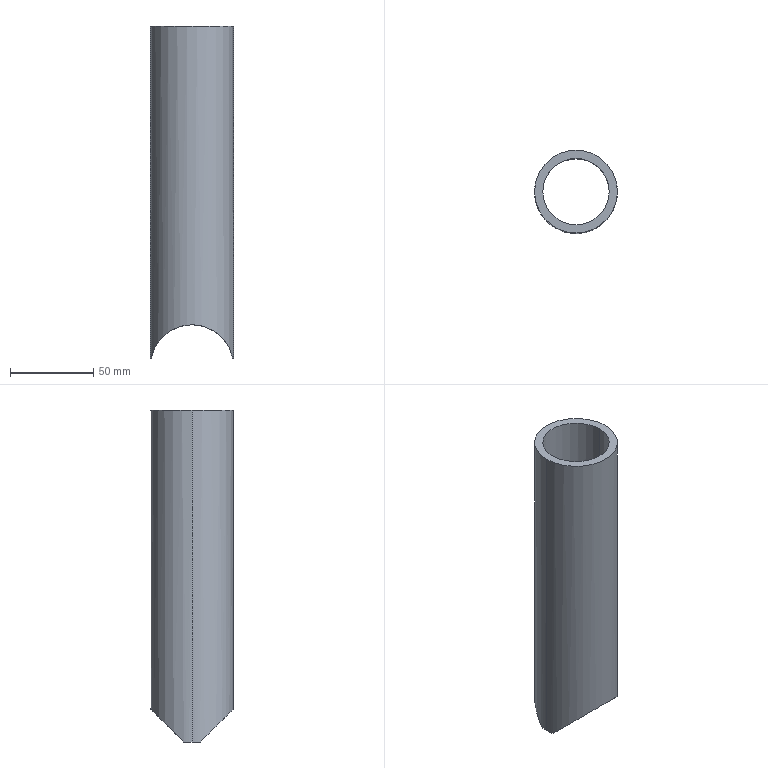Part | SolidWorks | features Extrusion 1, ICE 1, WeldmentFeature 1 | 1 solid | 8 faces | box 50 x 50 x 200 mm | volume 131874 mm3 | cylinder 5 | plane 3 | commonest cylinder face diameters 50 x3 40 x2
STEP:
#1=CARTESIAN_POINT('',(-20.,0.,200.));
#2=VERTEX_POINT('',#1);
#3=CARTESIAN_POINT('',(20.,0.,200.));
#4=VERTEX_POINT('',#3);
#5=CARTESIAN_POINT('',(0.,0.,200.));
#6=DIRECTION('',(0.,0.,1.));
#7=DIRECTION('',(1.,0.,0.));
#8=AXIS2_PLACEMENT_3D('',#5,#6,#7);
#9=CIRCLE('',#8,20.);
#10=EDGE_CURVE('',#2,#4,#9,.T.);
#11=ORIENTED_EDGE('',*,*,#10,.T.);
#12=CARTESIAN_POINT('',(20.,0.,10.));
#13=VERTEX_POINT('',#12);
#14=CARTESIAN_POINT('',(20.,0.,200.));
#15=DIRECTION('',(0.,0.,-1.));
#16=VECTOR('',#15,1000.);
#17=LINE('',#14,#16);
#18=EDGE_CURVE('',#4,#13,#17,.T.);
#19=ORIENTED_EDGE('',*,*,#18,.T.);
#20=CARTESIAN_POINT('',(-20.,0.,10.));
#21=VERTEX_POINT('',#20);
#22=CARTESIAN_POINT('',(20.,0.,10.));
#23=CARTESIAN_POINT('',(20.,-0.6946,10.));
#24=CARTESIAN_POINT('',(19.964,-1.383,10.048));
#25=CARTESIAN_POINT('',(19.858,-2.406,10.188));
#26=CARTESIAN_POINT('',(19.814,-2.745,10.246));
#27=CARTESIAN_POINT('',(19.708,-3.421,10.382));
#28=CARTESIAN_POINT('',(19.647,-3.758,10.46));
#29=CARTESIAN_POINT('',(19.302,-5.409,10.894));
#30=CARTESIAN_POINT('',(18.908,-6.644,11.372));
#31=CARTESIAN_POINT('',(18.158,-8.409,12.188));
#32=CARTESIAN_POINT('',(17.88,-8.983,12.478));
#33=CARTESIAN_POINT('',(17.283,-10.085,13.069));
#34=CARTESIAN_POINT('',(16.962,-10.615,13.372));
#35=CARTESIAN_POINT('',(15.932,-12.154,14.288));
#36=CARTESIAN_POINT('',(15.156,-13.109,14.91));
#37=CARTESIAN_POINT('',(13.845,-14.447,15.823));
#38=CARTESIAN_POINT('',(13.382,-14.877,16.124));
#39=CARTESIAN_POINT('',(12.423,-15.687,16.702));
#40=CARTESIAN_POINT('',(11.924,-16.069,16.981));
#41=CARTESIAN_POINT('',(10.366,-17.151,17.78));
#42=CARTESIAN_POINT('',(9.247,-17.784,18.263));
#43=CARTESIAN_POINT('',(7.725,-18.451,18.779));
#44=CARTESIAN_POINT('',(7.414,-18.578,18.878));
#45=CARTESIAN_POINT('',(6.785,-18.817,19.064));
#46=CARTESIAN_POINT('',(6.468,-18.928,19.151));
#47=CARTESIAN_POINT('',(5.505,-19.239,19.395));
#48=CARTESIAN_POINT('',(4.851,-19.415,19.534));
#49=CARTESIAN_POINT('',(3.517,-19.7,19.761));
#50=CARTESIAN_POINT('',(2.835,-19.81,19.848));
#51=CARTESIAN_POINT('',(1.447,-19.96,19.968));
#52=CARTESIAN_POINT('',(0.7543,-19.998,19.998));
#53=CARTESIAN_POINT('',(-0.6273,-20.002,20.002));
#54=CARTESIAN_POINT('',(-1.316,-19.969,19.975));
#55=CARTESIAN_POINT('',(-2.347,-19.865,19.892));
#56=CARTESIAN_POINT('',(-2.69,-19.821,19.857));
#57=CARTESIAN_POINT('',(-3.376,-19.716,19.773));
#58=CARTESIAN_POINT('',(-3.718,-19.654,19.724));
#59=CARTESIAN_POINT('',(-5.403,-19.306,19.447));
#60=CARTESIAN_POINT('',(-6.686,-18.897,19.124));
#61=CARTESIAN_POINT('',(-8.218,-18.237,18.613));
#62=CARTESIAN_POINT('',(-8.521,-18.097,18.505));
#63=CARTESIAN_POINT('',(-9.114,-17.806,18.282));
#64=CARTESIAN_POINT('',(-9.405,-17.654,18.166));
#65=CARTESIAN_POINT('',(-10.26,-17.18,17.806));
#66=CARTESIAN_POINT('',(-10.807,-16.841,17.551));
#67=CARTESIAN_POINT('',(-11.862,-16.116,17.015));
#68=CARTESIAN_POINT('',(-12.368,-15.73,16.734));
#69=CARTESIAN_POINT('',(-13.342,-14.913,16.15));
#70=CARTESIAN_POINT('',(-13.803,-14.487,15.851));
#71=CARTESIAN_POINT('',(-15.116,-13.156,14.941));
#72=CARTESIAN_POINT('',(-15.898,-12.199,14.316));
#73=CARTESIAN_POINT('',(-16.943,-10.646,13.389));
#74=CARTESIAN_POINT('',(-17.269,-10.107,13.082));
#75=CARTESIAN_POINT('',(-17.869,-9.004,12.489));
#76=CARTESIAN_POINT('',(-18.144,-8.437,12.202));
#77=CARTESIAN_POINT('',(-18.644,-7.267,11.659));
#78=CARTESIAN_POINT('',(-18.869,-6.664,11.403));
#79=CARTESIAN_POINT('',(-19.265,-5.413,10.936));
#80=CARTESIAN_POINT('',(-19.436,-4.763,10.725));
#81=CARTESIAN_POINT('',(-19.712,-3.446,10.378));
#82=CARTESIAN_POINT('',(-19.818,-2.775,10.239));
#83=CARTESIAN_POINT('',(-19.926,-1.748,10.098));
#84=CARTESIAN_POINT('',(-19.954,-1.403,10.061));
#85=CARTESIAN_POINT('',(-19.991,-0.7036,10.012));
#86=CARTESIAN_POINT('',(-20.,-0.3509,10.));
#87=CARTESIAN_POINT('',(-20.,0.,10.));
#88=B_SPLINE_CURVE_WITH_KNOTS('',3,(#22,#23,#24,#25,#26,#27,#28,#29,#30,#31,#32,#33,#34,#35,#36,#37,#38,#39,#40,#41,#42,#43,#44,#45,#46,#47,#48,#49,#50,#51,#52,#53,#54,#55,#56,#57,#58,#59,#60,#61,#62,#63,#64,#65,#66,#67,#68,#69,#70,#71,#72,#73,#74,#75,#76,#77,#78,#79,#80,#81,#82,#83,#84,#85,#86,#87),.UNSPECIFIED.,.F.,.F.,(4,2,2,2,2,2,2,2,2,2,2,2,2,2,2,2,2,2,2,2,2,2,2,2,2,2,2,2,2,2,2,2,4),(0.06633,0.0684,0.06944,0.07048,0.07462,0.07669,0.07876,0.0829,0.08497,0.08705,0.09119,0.09222,0.09326,0.09533,0.0974,0.09947,0.1015,0.1026,0.1036,0.1078,0.1088,0.1098,0.1119,0.114,0.116,0.1202,0.1223,0.1243,0.1264,0.1285,0.1305,0.1316,0.1326),.UNSPECIFIED.);
#89=EDGE_CURVE('',#13,#21,#88,.T.);
#90=ORIENTED_EDGE('',*,*,#89,.T.);
#91=CARTESIAN_POINT('',(-20.,0.,200.));
#92=DIRECTION('',(0.,0.,-1.));
#93=VECTOR('',#92,1000.);
#94=LINE('',#91,#93);
#95=EDGE_CURVE('',#2,#21,#94,.T.);
#96=ORIENTED_EDGE('',*,*,#95,.F.);
#97=EDGE_LOOP('',(#11,#19,#90,#96));
#98=FACE_OUTER_BOUND('',#97,.T.);
#99=CARTESIAN_POINT('',(0.,0.,200.));
#100=DIRECTION('',(0.,0.,-1.));
#101=DIRECTION('',(-1.,0.,0.));
#102=AXIS2_PLACEMENT_3D('',#99,#100,#101);
#103=CYLINDRICAL_SURFACE('',#102,20.);
#104=ADVANCED_FACE('',(#98),#103,.F.);
#105=CARTESIAN_POINT('',(25.,0.,200.));
#106=VERTEX_POINT('',#105);
#107=CARTESIAN_POINT('',(-25.,0.,200.));
#108=VERTEX_POINT('',#107);
#109=CARTESIAN_POINT('',(0.,0.,200.));
#110=DIRECTION('',(0.,0.,1.));
#111=DIRECTION('',(1.,0.,0.));
#112=AXIS2_PLACEMENT_3D('',#109,#110,#111);
#113=CIRCLE('',#112,25.);
#114=EDGE_CURVE('',#106,#108,#113,.T.);
#115=ORIENTED_EDGE('',*,*,#114,.F.);
#116=CARTESIAN_POINT('',(25.,0.,0.));
#117=VERTEX_POINT('',#116);
#118=CARTESIAN_POINT('',(25.,0.,200.));
#119=DIRECTION('',(0.,0.,-1.));
#120=VECTOR('',#119,1000.);
#121=LINE('',#118,#120);
#122=EDGE_CURVE('',#106,#117,#121,.T.);
#123=ORIENTED_EDGE('',*,*,#122,.T.);
#124=CARTESIAN_POINT('',(24.495,5.,0.));
#125=VERTEX_POINT('',#124);
#126=CARTESIAN_POINT('',(0.,0.,0.));
#127=DIRECTION('',(0.,0.,1.));
#128=DIRECTION('',(1.,0.,0.));
#129=AXIS2_PLACEMENT_3D('',#126,#127,#128);
#130=CIRCLE('',#129,25.);
#131=EDGE_CURVE('',#117,#125,#130,.T.);
#132=ORIENTED_EDGE('',*,*,#131,.T.);
#133=CARTESIAN_POINT('',(-24.495,5.,0.));
#134=VERTEX_POINT('',#133);
#135=CARTESIAN_POINT('',(-24.495,5.,0.));
#136=CARTESIAN_POINT('',(-17.496,39.286,34.286));
#137=CARTESIAN_POINT('',(17.496,39.286,34.286));
#138=CARTESIAN_POINT('',(24.495,5.,0.));
#139=(BOUNDED_CURVE()B_SPLINE_CURVE(3,(#135,#136,#137,#138),.UNSPECIFIED.,.F.,.F.)B_SPLINE_CURVE_WITH_KNOTS((4,4),(1.772,4.511),.UNSPECIFIED.)CURVE()GEOMETRIC_REPRESENTATION_ITEM()RATIONAL_B_SPLINE_CURVE((1.,0.4667,0.4667,1.))REPRESENTATION_ITEM(''));
#140=EDGE_CURVE('',#134,#125,#139,.T.);
#141=ORIENTED_EDGE('',*,*,#140,.F.);
#142=CARTESIAN_POINT('',(-25.,0.,0.));
#143=VERTEX_POINT('',#142);
#144=CARTESIAN_POINT('',(0.,0.,0.));
#145=DIRECTION('',(0.,0.,1.));
#146=DIRECTION('',(1.,0.,0.));
#147=AXIS2_PLACEMENT_3D('',#144,#145,#146);
#148=CIRCLE('',#147,25.);
#149=EDGE_CURVE('',#134,#143,#148,.T.);
#150=ORIENTED_EDGE('',*,*,#149,.T.);
#151=CARTESIAN_POINT('',(-25.,0.,200.));
#152=DIRECTION('',(0.,0.,-1.));
#153=VECTOR('',#152,1000.);
#154=LINE('',#151,#153);
#155=EDGE_CURVE('',#108,#143,#154,.T.);
#156=ORIENTED_EDGE('',*,*,#155,.F.);
#157=EDGE_LOOP('',(#115,#123,#132,#141,#150,#156));
#158=FACE_OUTER_BOUND('',#157,.T.);
#159=CARTESIAN_POINT('',(0.,0.,200.));
#160=DIRECTION('',(0.,0.,-1.));
#161=DIRECTION('',(-1.,0.,0.));
#162=AXIS2_PLACEMENT_3D('',#159,#160,#161);
#163=CYLINDRICAL_SURFACE('',#162,25.);
#164=ADVANCED_FACE('',(#158),#163,.T.);
#165=CARTESIAN_POINT('',(-24.495,-5.,0.));
#166=VERTEX_POINT('',#165);
#167=CARTESIAN_POINT('',(-24.495,500.,0.));
#168=DIRECTION('',(0.,1.,0.));
#169=VECTOR('',#168,1000.);
#170=LINE('',#167,#169);
#171=EDGE_CURVE('',#166,#134,#170,.T.);
#172=ORIENTED_EDGE('',*,*,#171,.F.);
#173=CARTESIAN_POINT('',(0.,0.,0.));
#174=DIRECTION('',(0.,0.,1.));
#175=DIRECTION('',(1.,0.,0.));
#176=AXIS2_PLACEMENT_3D('',#173,#174,#175);
#177=CIRCLE('',#176,25.);
#178=EDGE_CURVE('',#143,#166,#177,.T.);
#179=ORIENTED_EDGE('',*,*,#178,.F.);
#180=ORIENTED_EDGE('',*,*,#149,.F.);
#181=EDGE_LOOP('',(#172,#179,#180));
#182=FACE_OUTER_BOUND('',#181,.T.);
#183=CARTESIAN_POINT('',(0.,0.,0.));
#184=DIRECTION('',(0.,0.,1.));
#185=DIRECTION('',(1.,0.,0.));
#186=AXIS2_PLACEMENT_3D('',#183,#184,#185);
#187=PLANE('',#186);
#188=ADVANCED_FACE('',(#182),#187,.F.);
#189=CARTESIAN_POINT('',(24.495,-5.,0.));
#190=VERTEX_POINT('',#189);
#191=CARTESIAN_POINT('',(24.495,500.,0.));
#192=DIRECTION('',(0.,-1.,0.));
#193=VECTOR('',#192,1000.);
#194=LINE('',#191,#193);
#195=EDGE_CURVE('',#125,#190,#194,.T.);
#196=ORIENTED_EDGE('',*,*,#195,.F.);
#197=ORIENTED_EDGE('',*,*,#131,.F.);
#198=CARTESIAN_POINT('',(0.,0.,0.));
#199=DIRECTION('',(0.,0.,1.));
#200=DIRECTION('',(1.,0.,0.));
#201=AXIS2_PLACEMENT_3D('',#198,#199,#200);
#202=CIRCLE('',#201,25.);
#203=EDGE_CURVE('',#190,#117,#202,.T.);
#204=ORIENTED_EDGE('',*,*,#203,.F.);
#205=EDGE_LOOP('',(#196,#197,#204));
#206=FACE_OUTER_BOUND('',#205,.T.);
#207=CARTESIAN_POINT('',(0.,0.,0.));
#208=DIRECTION('',(0.,0.,1.));
#209=DIRECTION('',(1.,0.,0.));
#210=AXIS2_PLACEMENT_3D('',#207,#208,#209);
#211=PLANE('',#210);
#212=ADVANCED_FACE('',(#206),#211,.F.);
#213=ORIENTED_EDGE('',*,*,#122,.F.);
#214=CARTESIAN_POINT('',(0.,0.,200.));
#215=DIRECTION('',(0.,0.,1.));
#216=DIRECTION('',(1.,0.,0.));
#217=AXIS2_PLACEMENT_3D('',#214,#215,#216);
#218=CIRCLE('',#217,25.);
#219=EDGE_CURVE('',#108,#106,#218,.T.);
#220=ORIENTED_EDGE('',*,*,#219,.F.);
#221=ORIENTED_EDGE('',*,*,#155,.T.);
#222=ORIENTED_EDGE('',*,*,#178,.T.);
#223=CARTESIAN_POINT('',(24.495,-5.,0.));
#224=CARTESIAN_POINT('',(17.496,-39.286,34.286));
#225=CARTESIAN_POINT('',(-17.496,-39.286,34.286));
#226=CARTESIAN_POINT('',(-24.495,-5.,0.));
#227=(BOUNDED_CURVE()B_SPLINE_CURVE(3,(#223,#224,#225,#226),.UNSPECIFIED.,.F.,.T.)B_SPLINE_CURVE_WITH_KNOTS((4,4),(1.772,4.511),.UNSPECIFIED.)CURVE()GEOMETRIC_REPRESENTATION_ITEM()RATIONAL_B_SPLINE_CURVE((1.,0.4667,0.4667,1.))REPRESENTATION_ITEM(''));
#228=EDGE_CURVE('',#190,#166,#227,.T.);
#229=ORIENTED_EDGE('',*,*,#228,.F.);
#230=ORIENTED_EDGE('',*,*,#203,.T.);
#231=EDGE_LOOP('',(#213,#220,#221,#222,#229,#230));
#232=FACE_OUTER_BOUND('',#231,.T.);
#233=CARTESIAN_POINT('',(0.,0.,200.));
#234=DIRECTION('',(0.,0.,-1.));
#235=DIRECTION('',(-1.,0.,0.));
#236=AXIS2_PLACEMENT_3D('',#233,#234,#235);
#237=CYLINDRICAL_SURFACE('',#236,25.);
#238=ADVANCED_FACE('',(#232),#237,.T.);
#239=ORIENTED_EDGE('',*,*,#18,.F.);
#240=CARTESIAN_POINT('',(0.,0.,200.));
#241=DIRECTION('',(0.,0.,1.));
#242=DIRECTION('',(1.,0.,0.));
#243=AXIS2_PLACEMENT_3D('',#240,#241,#242);
#244=CIRCLE('',#243,20.);
#245=EDGE_CURVE('',#4,#2,#244,.T.);
#246=ORIENTED_EDGE('',*,*,#245,.T.);
#247=ORIENTED_EDGE('',*,*,#95,.T.);
#248=CARTESIAN_POINT('',(-20.,0.,10.));
#249=CARTESIAN_POINT('',(-20.,1.405,10.));
#250=CARTESIAN_POINT('',(-19.854,2.765,10.199));
#251=CARTESIAN_POINT('',(-19.509,4.419,10.634));
#252=CARTESIAN_POINT('',(-19.431,4.748,10.73));
#253=CARTESIAN_POINT('',(-19.263,5.391,10.936));
#254=CARTESIAN_POINT('',(-19.171,5.707,11.046));
#255=CARTESIAN_POINT('',(-18.877,6.639,11.394));
#256=CARTESIAN_POINT('',(-18.654,7.241,11.648));
#257=CARTESIAN_POINT('',(-18.156,8.412,12.19));
#258=CARTESIAN_POINT('',(-17.882,8.98,12.476));
#259=CARTESIAN_POINT('',(-17.281,10.089,13.071));
#260=CARTESIAN_POINT('',(-16.957,10.624,13.376));
#261=CARTESIAN_POINT('',(-15.922,12.167,14.296));
#262=CARTESIAN_POINT('',(-15.147,13.119,14.917));
#263=CARTESIAN_POINT('',(-13.844,14.448,15.824));
#264=CARTESIAN_POINT('',(-13.386,14.873,16.122));
#265=CARTESIAN_POINT('',(-12.418,15.69,16.705));
#266=CARTESIAN_POINT('',(-11.913,16.078,16.987));
#267=CARTESIAN_POINT('',(-10.341,17.167,17.792));
#268=CARTESIAN_POINT('',(-9.215,17.8,18.275));
#269=CARTESIAN_POINT('',(-7.692,18.465,18.79));
#270=CARTESIAN_POINT('',(-7.38,18.592,18.888));
#271=CARTESIAN_POINT('',(-6.751,18.829,19.073));
#272=CARTESIAN_POINT('',(-6.433,18.94,19.16));
#273=CARTESIAN_POINT('',(-5.471,19.249,19.403));
#274=CARTESIAN_POINT('',(-4.817,19.423,19.541));
#275=CARTESIAN_POINT('',(-3.483,19.706,19.765));
#276=CARTESIAN_POINT('',(-2.803,19.815,19.852));
#277=CARTESIAN_POINT('',(-1.415,19.962,19.97));
#278=CARTESIAN_POINT('',(-0.7219,19.999,19.999));
#279=CARTESIAN_POINT('',(0.6588,20.001,20.001));
#280=CARTESIAN_POINT('',(1.347,19.967,19.973));
#281=CARTESIAN_POINT('',(2.376,19.861,19.889));
#282=CARTESIAN_POINT('',(2.719,19.817,19.854));
#283=CARTESIAN_POINT('',(3.403,19.711,19.77));
#284=CARTESIAN_POINT('',(3.745,19.649,19.72));
#285=CARTESIAN_POINT('',(5.428,19.298,19.442));
#286=CARTESIAN_POINT('',(6.71,18.888,19.117));
#287=CARTESIAN_POINT('',(8.239,18.227,18.606));
#288=CARTESIAN_POINT('',(8.541,18.087,18.498));
#289=CARTESIAN_POINT('',(9.134,17.796,18.274));
#290=CARTESIAN_POINT('',(9.424,17.644,18.158));
#291=CARTESIAN_POINT('',(10.278,17.17,17.798));
#292=CARTESIAN_POINT('',(10.824,16.83,17.543));
#293=CARTESIAN_POINT('',(11.877,16.105,17.007));
#294=CARTESIAN_POINT('',(12.382,15.719,16.726));
#295=CARTESIAN_POINT('',(13.354,14.903,16.142));
#296=CARTESIAN_POINT('',(13.815,14.476,15.843));
#297=CARTESIAN_POINT('',(15.125,13.144,14.934));
#298=CARTESIAN_POINT('',(15.906,12.188,14.31));
#299=CARTESIAN_POINT('',(16.949,10.636,13.384));
#300=CARTESIAN_POINT('',(17.275,10.098,13.076));
#301=CARTESIAN_POINT('',(17.874,8.995,12.484));
#302=CARTESIAN_POINT('',(18.149,8.428,12.198));
#303=CARTESIAN_POINT('',(18.648,7.258,11.656));
#304=CARTESIAN_POINT('',(18.872,6.655,11.4));
#305=CARTESIAN_POINT('',(19.267,5.406,10.934));
#306=CARTESIAN_POINT('',(19.438,4.756,10.723));
#307=CARTESIAN_POINT('',(19.714,3.439,10.376));
#308=CARTESIAN_POINT('',(19.819,2.768,10.238));
#309=CARTESIAN_POINT('',(19.927,1.742,10.097));
#310=CARTESIAN_POINT('',(19.954,1.397,10.061));
#311=CARTESIAN_POINT('',(19.991,0.698,10.012));
#312=CARTESIAN_POINT('',(20.,0.3476,10.));
#313=CARTESIAN_POINT('',(20.,0.,10.));
#314=B_SPLINE_CURVE_WITH_KNOTS('',3,(#248,#249,#250,#251,#252,#253,#254,#255,#256,#257,#258,#259,#260,#261,#262,#263,#264,#265,#266,#267,#268,#269,#270,#271,#272,#273,#274,#275,#276,#277,#278,#279,#280,#281,#282,#283,#284,#285,#286,#287,#288,#289,#290,#291,#292,#293,#294,#295,#296,#297,#298,#299,#300,#301,#302,#303,#304,#305,#306,#307,#308,#309,#310,#311,#312,#313),.UNSPECIFIED.,.F.,.F.,(4,2,2,2,2,2,2,2,2,2,2,2,2,2,2,2,2,2,2,2,2,2,2,2,2,2,2,2,2,2,2,2,4),(0.,0.004146,0.005182,0.006219,0.008292,0.01036,0.01244,0.01658,0.01866,0.02073,0.02487,0.02591,0.02695,0.02902,0.03109,0.03317,0.03524,0.03628,0.03731,0.04146,0.04249,0.04353,0.0456,0.04768,0.04975,0.0539,0.05597,0.05804,0.06011,0.06219,0.06426,0.0653,0.06633),.UNSPECIFIED.);
#315=EDGE_CURVE('',#21,#13,#314,.T.);
#316=ORIENTED_EDGE('',*,*,#315,.T.);
#317=EDGE_LOOP('',(#239,#246,#247,#316));
#318=FACE_OUTER_BOUND('',#317,.T.);
#319=CARTESIAN_POINT('',(0.,0.,200.));
#320=DIRECTION('',(0.,0.,-1.));
#321=DIRECTION('',(-1.,0.,0.));
#322=AXIS2_PLACEMENT_3D('',#319,#320,#321);
#323=CYLINDRICAL_SURFACE('',#322,20.);
#324=ADVANCED_FACE('',(#318),#323,.F.);
#325=ORIENTED_EDGE('',*,*,#219,.T.);
#326=ORIENTED_EDGE('',*,*,#114,.T.);
#327=EDGE_LOOP('',(#325,#326));
#328=FACE_OUTER_BOUND('',#327,.T.);
#329=ORIENTED_EDGE('',*,*,#10,.F.);
#330=ORIENTED_EDGE('',*,*,#245,.F.);
#331=EDGE_LOOP('',(#329,#330));
#332=FACE_BOUND('',#331,.T.);
#333=CARTESIAN_POINT('',(0.,0.,200.));
#334=DIRECTION('',(0.,0.,1.));
#335=DIRECTION('',(1.,0.,0.));
#336=AXIS2_PLACEMENT_3D('',#333,#334,#335);
#337=PLANE('',#336);
#338=ADVANCED_FACE('',(#328,#332),#337,.T.);
#339=ORIENTED_EDGE('',*,*,#315,.F.);
#340=ORIENTED_EDGE('',*,*,#89,.F.);
#341=EDGE_LOOP('',(#339,#340));
#342=FACE_BOUND('',#341,.T.);
#343=ORIENTED_EDGE('',*,*,#228,.T.);
#344=ORIENTED_EDGE('',*,*,#171,.T.);
#345=ORIENTED_EDGE('',*,*,#140,.T.);
#346=ORIENTED_EDGE('',*,*,#195,.T.);
#347=EDGE_LOOP('',(#343,#344,#345,#346));
#348=FACE_OUTER_BOUND('',#347,.T.);
#349=CARTESIAN_POINT('',(0.,500.,-5.));
#350=DIRECTION('',(0.,-1.,0.));
#351=DIRECTION('',(0.,0.,-1.));
#352=AXIS2_PLACEMENT_3D('',#349,#350,#351);
#353=CYLINDRICAL_SURFACE('',#352,25.);
#354=ADVANCED_FACE('',(#342,#348),#353,.F.);
#355=CLOSED_SHELL('',(#104,#164,#188,#212,#238,#324,#338,#354));
#356=MANIFOLD_SOLID_BREP('',#355);
#357=CARTESIAN_POINT('',(0.,0.,0.));
#358=DIRECTION('',(0.,0.,1.));
#359=DIRECTION('',(1.,0.,0.));
#360=AXIS2_PLACEMENT_3D('',#357,#358,#359);
#361=(LENGTH_UNIT()NAMED_UNIT(*)SI_UNIT(.MILLI.,.METRE.));
#362=UNCERTAINTY_MEASURE_WITH_UNIT(LENGTH_MEASURE(0.00001),#361,'','');
#363=(NAMED_UNIT(*)PLANE_ANGLE_UNIT()SI_UNIT($,.RADIAN.));
#364=(NAMED_UNIT(*)SI_UNIT($,.STERADIAN.)SOLID_ANGLE_UNIT());
#365=(GEOMETRIC_REPRESENTATION_CONTEXT(3)GLOBAL_UNCERTAINTY_ASSIGNED_CONTEXT((#362))GLOBAL_UNIT_ASSIGNED_CONTEXT((#361,#363,#364))REPRESENTATION_CONTEXT('',''));
#366=ADVANCED_BREP_SHAPE_REPRESENTATION('',(#356,#360),#365);